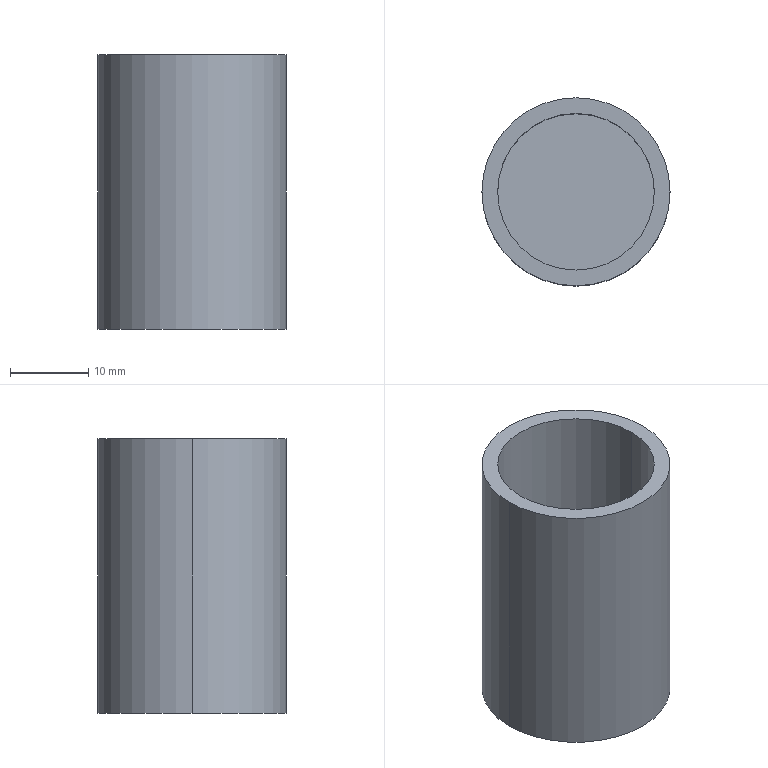Part | STEP file | end shield | 1 solid | 7 faces | box 24 x 24 x 35 mm | volume 6409 mm3 | cylinder 4 | plane 3 | commonest cylinder face diameters 20 x2 24 x2
STEP:
#1=CARTESIAN_POINT('',(-10.,0.,5.));
#2=VERTEX_POINT('',#1);
#3=CARTESIAN_POINT('',(10.,0.,5.));
#4=VERTEX_POINT('',#3);
#5=CARTESIAN_POINT('',(0.,0.,5.));
#6=DIRECTION('',(0.,0.,1.));
#7=DIRECTION('',(1.,0.,0.));
#8=AXIS2_PLACEMENT_3D('',#5,#6,#7);
#9=CIRCLE('',#8,10.);
#10=EDGE_CURVE('',#2,#4,#9,.T.);
#11=ORIENTED_EDGE('',*,*,#10,.F.);
#12=CARTESIAN_POINT('',(-10.,0.,35.));
#13=VERTEX_POINT('',#12);
#14=CARTESIAN_POINT('',(-10.,0.,5.));
#15=DIRECTION('',(0.,0.,1.));
#16=VECTOR('',#15,1000.);
#17=LINE('',#14,#16);
#18=EDGE_CURVE('',#2,#13,#17,.T.);
#19=ORIENTED_EDGE('',*,*,#18,.T.);
#20=CARTESIAN_POINT('',(10.,0.,35.));
#21=VERTEX_POINT('',#20);
#22=CARTESIAN_POINT('',(0.,0.,35.));
#23=DIRECTION('',(0.,0.,1.));
#24=DIRECTION('',(1.,0.,0.));
#25=AXIS2_PLACEMENT_3D('',#22,#23,#24);
#26=CIRCLE('',#25,10.);
#27=EDGE_CURVE('',#13,#21,#26,.T.);
#28=ORIENTED_EDGE('',*,*,#27,.T.);
#29=CARTESIAN_POINT('',(10.,0.,5.));
#30=DIRECTION('',(0.,0.,1.));
#31=VECTOR('',#30,1000.);
#32=LINE('',#29,#31);
#33=EDGE_CURVE('',#4,#21,#32,.T.);
#34=ORIENTED_EDGE('',*,*,#33,.F.);
#35=EDGE_LOOP('',(#11,#19,#28,#34));
#36=FACE_OUTER_BOUND('',#35,.T.);
#37=CARTESIAN_POINT('',(0.,0.,5.));
#38=DIRECTION('',(0.,0.,1.));
#39=DIRECTION('',(1.,0.,0.));
#40=AXIS2_PLACEMENT_3D('',#37,#38,#39);
#41=CYLINDRICAL_SURFACE('',#40,10.);
#42=ADVANCED_FACE('',(#36),#41,.F.);
#43=CARTESIAN_POINT('',(12.,0.,35.));
#44=VERTEX_POINT('',#43);
#45=CARTESIAN_POINT('',(-12.,0.,35.));
#46=VERTEX_POINT('',#45);
#47=CARTESIAN_POINT('',(0.,0.,35.));
#48=DIRECTION('',(0.,0.,1.));
#49=DIRECTION('',(1.,0.,0.));
#50=AXIS2_PLACEMENT_3D('',#47,#48,#49);
#51=CIRCLE('',#50,12.);
#52=EDGE_CURVE('',#44,#46,#51,.T.);
#53=ORIENTED_EDGE('',*,*,#52,.F.);
#54=CARTESIAN_POINT('',(12.,0.,0.));
#55=VERTEX_POINT('',#54);
#56=CARTESIAN_POINT('',(12.,0.,35.));
#57=DIRECTION('',(0.,0.,-1.));
#58=VECTOR('',#57,1000.);
#59=LINE('',#56,#58);
#60=EDGE_CURVE('',#44,#55,#59,.T.);
#61=ORIENTED_EDGE('',*,*,#60,.T.);
#62=CARTESIAN_POINT('',(-12.,0.,0.));
#63=VERTEX_POINT('',#62);
#64=CARTESIAN_POINT('',(0.,0.,0.));
#65=DIRECTION('',(0.,0.,1.));
#66=DIRECTION('',(1.,0.,0.));
#67=AXIS2_PLACEMENT_3D('',#64,#65,#66);
#68=CIRCLE('',#67,12.);
#69=EDGE_CURVE('',#55,#63,#68,.T.);
#70=ORIENTED_EDGE('',*,*,#69,.T.);
#71=CARTESIAN_POINT('',(-12.,0.,35.));
#72=DIRECTION('',(0.,0.,-1.));
#73=VECTOR('',#72,1000.);
#74=LINE('',#71,#73);
#75=EDGE_CURVE('',#46,#63,#74,.T.);
#76=ORIENTED_EDGE('',*,*,#75,.F.);
#77=EDGE_LOOP('',(#53,#61,#70,#76));
#78=FACE_OUTER_BOUND('',#77,.T.);
#79=CARTESIAN_POINT('',(0.,0.,35.));
#80=DIRECTION('',(0.,0.,-1.));
#81=DIRECTION('',(-1.,0.,0.));
#82=AXIS2_PLACEMENT_3D('',#79,#80,#81);
#83=CYLINDRICAL_SURFACE('',#82,12.);
#84=ADVANCED_FACE('',(#78),#83,.T.);
#85=ORIENTED_EDGE('',*,*,#60,.F.);
#86=CARTESIAN_POINT('',(0.,0.,35.));
#87=DIRECTION('',(0.,0.,1.));
#88=DIRECTION('',(1.,0.,0.));
#89=AXIS2_PLACEMENT_3D('',#86,#87,#88);
#90=CIRCLE('',#89,12.);
#91=EDGE_CURVE('',#46,#44,#90,.T.);
#92=ORIENTED_EDGE('',*,*,#91,.F.);
#93=ORIENTED_EDGE('',*,*,#75,.T.);
#94=CARTESIAN_POINT('',(0.,0.,0.));
#95=DIRECTION('',(0.,0.,1.));
#96=DIRECTION('',(1.,0.,0.));
#97=AXIS2_PLACEMENT_3D('',#94,#95,#96);
#98=CIRCLE('',#97,12.);
#99=EDGE_CURVE('',#63,#55,#98,.T.);
#100=ORIENTED_EDGE('',*,*,#99,.T.);
#101=EDGE_LOOP('',(#85,#92,#93,#100));
#102=FACE_OUTER_BOUND('',#101,.T.);
#103=CARTESIAN_POINT('',(0.,0.,35.));
#104=DIRECTION('',(0.,0.,-1.));
#105=DIRECTION('',(-1.,0.,0.));
#106=AXIS2_PLACEMENT_3D('',#103,#104,#105);
#107=CYLINDRICAL_SURFACE('',#106,12.);
#108=ADVANCED_FACE('',(#102),#107,.T.);
#109=CARTESIAN_POINT('',(0.,0.,35.));
#110=DIRECTION('',(0.,0.,1.));
#111=DIRECTION('',(1.,0.,0.));
#112=AXIS2_PLACEMENT_3D('',#109,#110,#111);
#113=CIRCLE('',#112,10.);
#114=EDGE_CURVE('',#21,#13,#113,.T.);
#115=ORIENTED_EDGE('',*,*,#114,.F.);
#116=ORIENTED_EDGE('',*,*,#27,.F.);
#117=EDGE_LOOP('',(#115,#116));
#118=FACE_BOUND('',#117,.T.);
#119=ORIENTED_EDGE('',*,*,#91,.T.);
#120=ORIENTED_EDGE('',*,*,#52,.T.);
#121=EDGE_LOOP('',(#119,#120));
#122=FACE_OUTER_BOUND('',#121,.T.);
#123=CARTESIAN_POINT('',(0.,0.,35.));
#124=DIRECTION('',(0.,0.,1.));
#125=DIRECTION('',(1.,0.,0.));
#126=AXIS2_PLACEMENT_3D('',#123,#124,#125);
#127=PLANE('',#126);
#128=ADVANCED_FACE('',(#118,#122),#127,.T.);
#129=ORIENTED_EDGE('',*,*,#99,.F.);
#130=ORIENTED_EDGE('',*,*,#69,.F.);
#131=EDGE_LOOP('',(#129,#130));
#132=FACE_OUTER_BOUND('',#131,.T.);
#133=CARTESIAN_POINT('',(0.,0.,0.));
#134=DIRECTION('',(0.,0.,1.));
#135=DIRECTION('',(1.,0.,0.));
#136=AXIS2_PLACEMENT_3D('',#133,#134,#135);
#137=PLANE('',#136);
#138=ADVANCED_FACE('',(#132),#137,.F.);
#139=ORIENTED_EDGE('',*,*,#18,.F.);
#140=CARTESIAN_POINT('',(0.,0.,5.));
#141=DIRECTION('',(0.,0.,1.));
#142=DIRECTION('',(1.,0.,0.));
#143=AXIS2_PLACEMENT_3D('',#140,#141,#142);
#144=CIRCLE('',#143,10.);
#145=EDGE_CURVE('',#4,#2,#144,.T.);
#146=ORIENTED_EDGE('',*,*,#145,.F.);
#147=ORIENTED_EDGE('',*,*,#33,.T.);
#148=ORIENTED_EDGE('',*,*,#114,.T.);
#149=EDGE_LOOP('',(#139,#146,#147,#148));
#150=FACE_OUTER_BOUND('',#149,.T.);
#151=CARTESIAN_POINT('',(0.,0.,5.));
#152=DIRECTION('',(0.,0.,1.));
#153=DIRECTION('',(1.,0.,0.));
#154=AXIS2_PLACEMENT_3D('',#151,#152,#153);
#155=CYLINDRICAL_SURFACE('',#154,10.);
#156=ADVANCED_FACE('',(#150),#155,.F.);
#157=ORIENTED_EDGE('',*,*,#145,.T.);
#158=ORIENTED_EDGE('',*,*,#10,.T.);
#159=EDGE_LOOP('',(#157,#158));
#160=FACE_OUTER_BOUND('',#159,.T.);
#161=CARTESIAN_POINT('',(0.,0.,5.));
#162=DIRECTION('',(0.,0.,1.));
#163=DIRECTION('',(1.,0.,0.));
#164=AXIS2_PLACEMENT_3D('',#161,#162,#163);
#165=PLANE('',#164);
#166=ADVANCED_FACE('',(#160),#165,.T.);
#167=CLOSED_SHELL('',(#42,#84,#108,#128,#138,#156,#166));
#168=MANIFOLD_SOLID_BREP('',#167);
#169=CARTESIAN_POINT('',(0.,0.,0.));
#170=DIRECTION('',(0.,0.,1.));
#171=DIRECTION('',(1.,0.,0.));
#172=AXIS2_PLACEMENT_3D('',#169,#170,#171);
#173=(LENGTH_UNIT()NAMED_UNIT(*)SI_UNIT(.MILLI.,.METRE.));
#174=UNCERTAINTY_MEASURE_WITH_UNIT(LENGTH_MEASURE(0.00001),#173,'','');
#175=(NAMED_UNIT(*)PLANE_ANGLE_UNIT()SI_UNIT($,.RADIAN.));
#176=(NAMED_UNIT(*)SI_UNIT($,.STERADIAN.)SOLID_ANGLE_UNIT());
#177=(GEOMETRIC_REPRESENTATION_CONTEXT(3)GLOBAL_UNCERTAINTY_ASSIGNED_CONTEXT((#174))GLOBAL_UNIT_ASSIGNED_CONTEXT((#173,#175,#176))REPRESENTATION_CONTEXT('',''));
#178=ADVANCED_BREP_SHAPE_REPRESENTATION('',(#168,#172),#177);